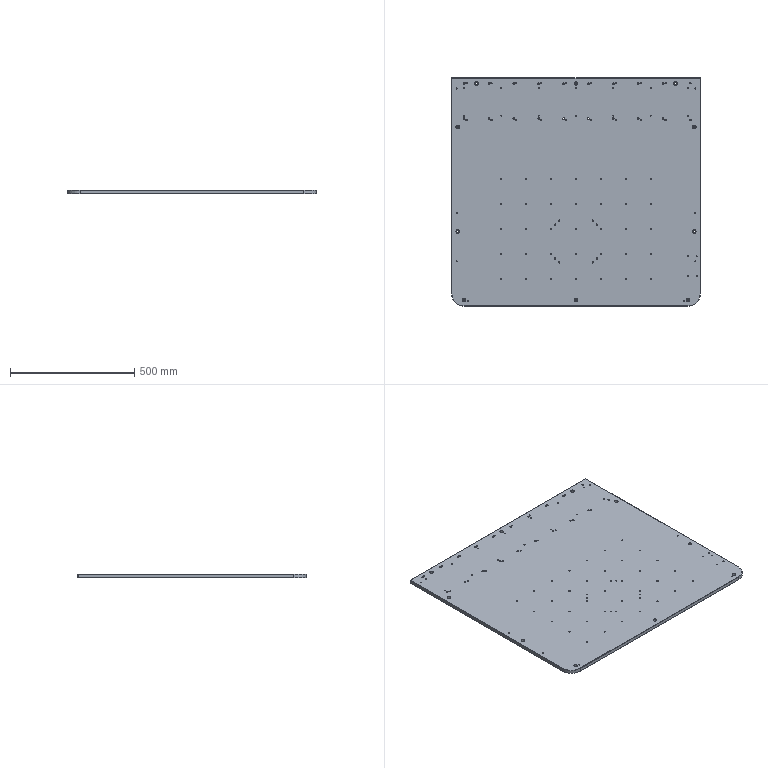Part | STEP file | FHD-021-015 H1010 revised work panel | 1 solid | 169 faces | box 1000 x 918 x 15 mm | volume 13697706 mm3 | cylinder 129 | plane 26 | cone 14 | commonest cylinder face diameters 5 x63 4.2 x26 6.8 x18 9 x10 14 x10 100 x2